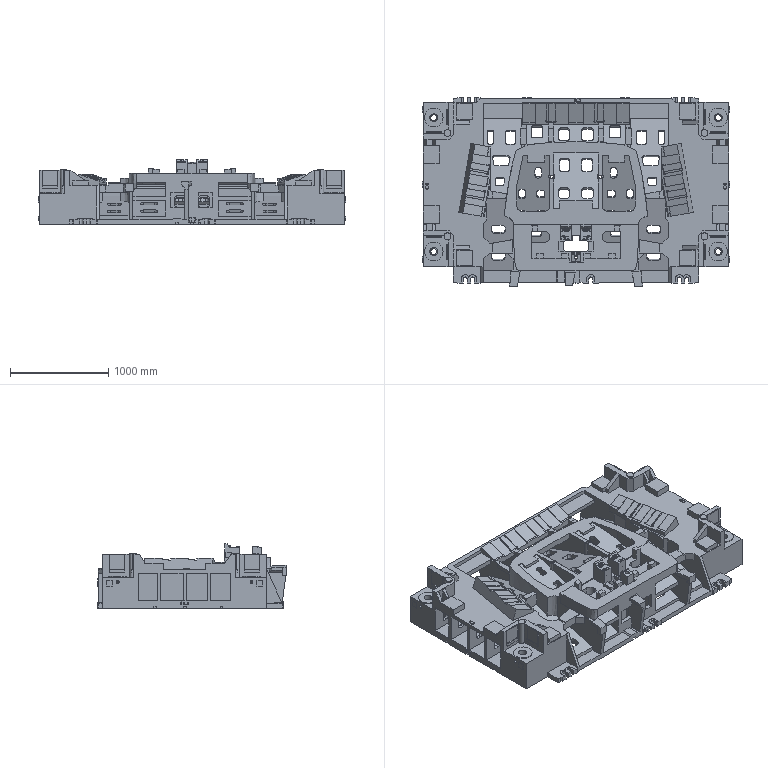Part | NX | features solid 2 | 1 solid | 2215 faces | box 3120 x 1920 x 656.008 mm | volume 850748358 mm3 | plane 1598 | cylinder 396 | spline 219 | cone 2 | commonest cylinder face diameters 50 x92 40 x81 60 x78 80 x40 20 x18 30 x14